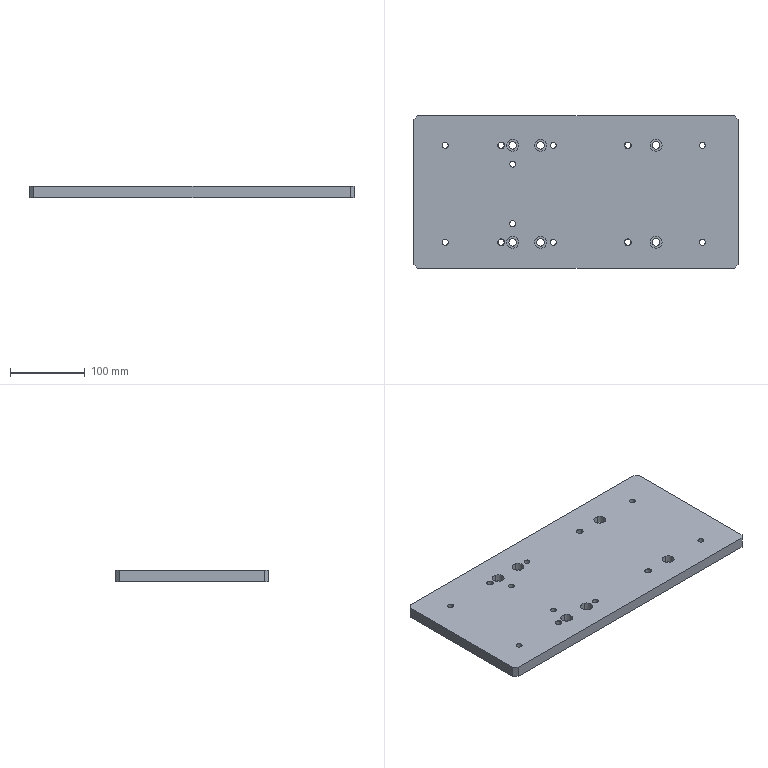Part | STEP file | J453-EBZ05-02-04-Part-1 | 1 solid | 90 faces | box 435 x 205 x 15 mm | volume 1311167 mm3 | cylinder 56 | plane 18 | cone 16 | commonest cylinder face diameters 8 x28 10 x12 16 x12 6.9 x4